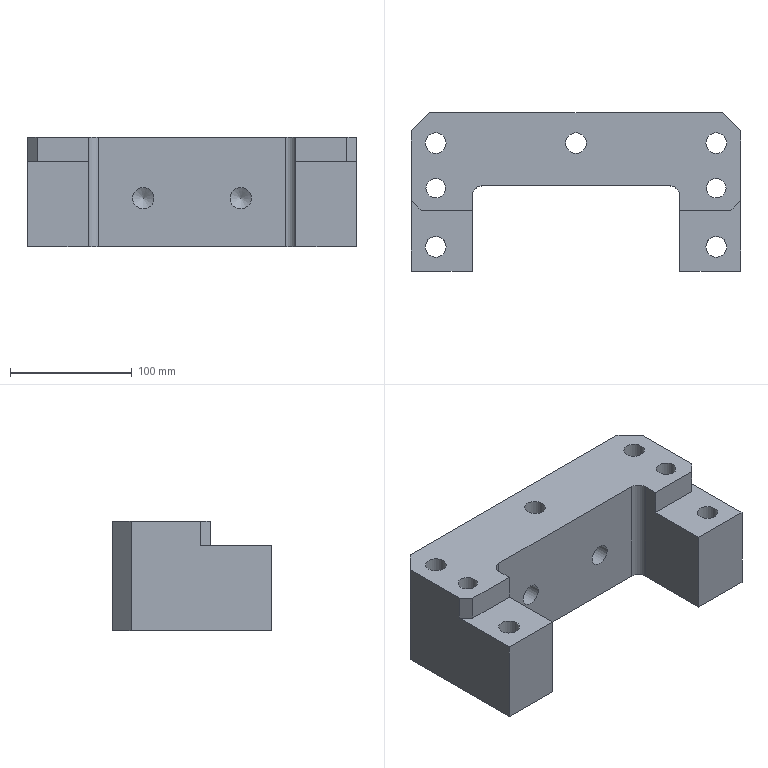Part | STEP file | 121_id150_x_t | 1 solid | 49 faces | box 270 x 130 x 90 mm | volume 1732261 mm3 | plane 25 | cylinder 20 | cone 4 | commonest cylinder face diameters 17 x5 26 x5 16 x4 14 x2 17.5 x2 18 x2